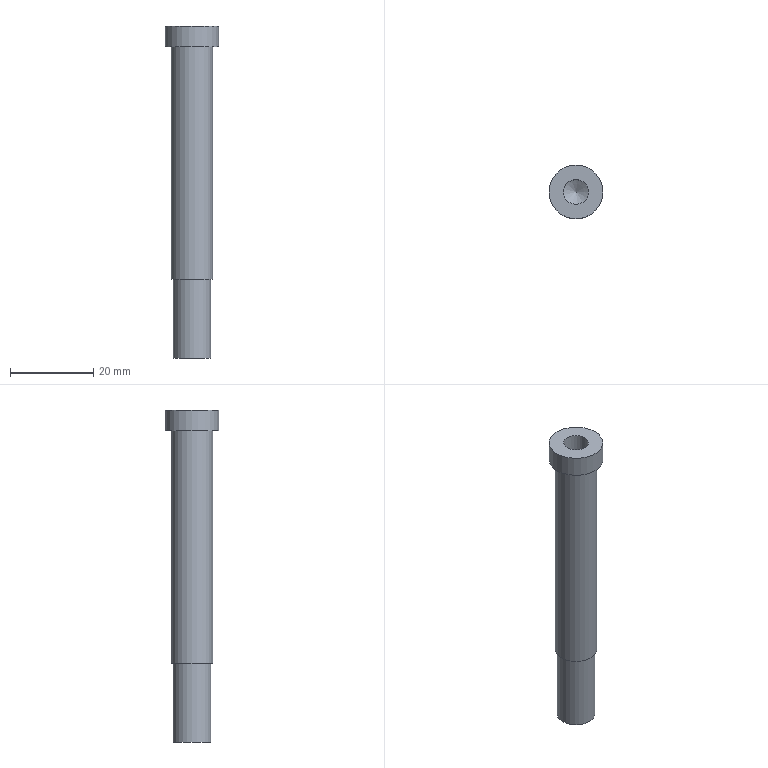Part | NX | features solid 2 | 1 solid | 9 faces | box 13 x 13 x 80 mm | volume 5914 mm3 | cylinder 4 | plane 4 | cone 1 | commonest cylinder face diameters 6 x1 9.1 x1 10 x1 13 x1
STEP:
#1=CARTESIAN_POINT('',(-691.699,-242.049,44.));
#2=VERTEX_POINT('',#1);
#3=CARTESIAN_POINT('',(-696.699,-242.049,44.));
#4=DIRECTION('',(0.,0.,1.));
#5=DIRECTION('',(1.,0.,0.));
#6=AXIS2_PLACEMENT_3D('',#3,#4,#5);
#7=CIRCLE('',#6,5.);
#8=EDGE_CURVE('',#2,#2,#7,.T.);
#9=ORIENTED_EDGE('',*,*,#8,.T.);
#10=EDGE_LOOP('',(#9));
#11=FACE_BOUND('',#10,.T.);
#12=CARTESIAN_POINT('',(-691.699,-242.049,100.));
#13=VERTEX_POINT('',#12);
#14=CARTESIAN_POINT('',(-696.699,-242.049,100.));
#15=DIRECTION('',(0.,0.,1.));
#16=DIRECTION('',(1.,0.,0.));
#17=AXIS2_PLACEMENT_3D('',#14,#15,#16);
#18=CIRCLE('',#17,5.);
#19=EDGE_CURVE('',#13,#13,#18,.T.);
#20=ORIENTED_EDGE('',*,*,#19,.F.);
#21=EDGE_LOOP('',(#20));
#22=FACE_BOUND('',#21,.T.);
#23=CARTESIAN_POINT('',(-696.699,-242.049,105.));
#24=DIRECTION('',(0.,0.,-1.));
#25=DIRECTION('',(-1.,0.,0.));
#26=AXIS2_PLACEMENT_3D('',#23,#24,#25);
#27=CYLINDRICAL_SURFACE('',#26,5.);
#28=ADVANCED_FACE('',(#11,#22),#27,.T.);
#29=CARTESIAN_POINT('',(-692.149,-242.049,44.));
#30=VERTEX_POINT('',#29);
#31=CARTESIAN_POINT('',(-696.699,-242.049,44.));
#32=DIRECTION('',(0.,0.,1.));
#33=DIRECTION('',(1.,0.,0.));
#34=AXIS2_PLACEMENT_3D('',#31,#32,#33);
#35=CIRCLE('',#34,4.55);
#36=EDGE_CURVE('',#30,#30,#35,.T.);
#37=ORIENTED_EDGE('',*,*,#36,.T.);
#38=EDGE_LOOP('',(#37));
#39=FACE_BOUND('',#38,.T.);
#40=ORIENTED_EDGE('',*,*,#8,.F.);
#41=EDGE_LOOP('',(#40));
#42=FACE_BOUND('',#41,.T.);
#43=CARTESIAN_POINT('',(-696.699,-242.049,44.));
#44=DIRECTION('',(0.,0.,1.));
#45=DIRECTION('',(1.,0.,0.));
#46=AXIS2_PLACEMENT_3D('',#43,#44,#45);
#47=PLANE('',#46);
#48=ADVANCED_FACE('',(#39,#42),#47,.F.);
#49=CARTESIAN_POINT('',(-690.199,-242.049,100.));
#50=VERTEX_POINT('',#49);
#51=CARTESIAN_POINT('',(-696.699,-242.049,100.));
#52=DIRECTION('',(0.,0.,1.));
#53=DIRECTION('',(1.,0.,0.));
#54=AXIS2_PLACEMENT_3D('',#51,#52,#53);
#55=CIRCLE('',#54,6.5);
#56=EDGE_CURVE('',#50,#50,#55,.T.);
#57=ORIENTED_EDGE('',*,*,#56,.F.);
#58=EDGE_LOOP('',(#57));
#59=FACE_BOUND('',#58,.T.);
#60=ORIENTED_EDGE('',*,*,#19,.T.);
#61=EDGE_LOOP('',(#60));
#62=FACE_BOUND('',#61,.T.);
#63=CARTESIAN_POINT('',(-696.699,-242.049,100.));
#64=DIRECTION('',(0.,0.,1.));
#65=DIRECTION('',(1.,0.,0.));
#66=AXIS2_PLACEMENT_3D('',#63,#64,#65);
#67=PLANE('',#66);
#68=ADVANCED_FACE('',(#59,#62),#67,.F.);
#69=ORIENTED_EDGE('',*,*,#56,.T.);
#70=EDGE_LOOP('',(#69));
#71=FACE_BOUND('',#70,.T.);
#72=CARTESIAN_POINT('',(-690.199,-242.049,105.));
#73=VERTEX_POINT('',#72);
#74=CARTESIAN_POINT('',(-696.699,-242.049,105.));
#75=DIRECTION('',(0.,0.,1.));
#76=DIRECTION('',(1.,0.,0.));
#77=AXIS2_PLACEMENT_3D('',#74,#75,#76);
#78=CIRCLE('',#77,6.5);
#79=EDGE_CURVE('',#73,#73,#78,.T.);
#80=ORIENTED_EDGE('',*,*,#79,.F.);
#81=EDGE_LOOP('',(#80));
#82=FACE_BOUND('',#81,.T.);
#83=CARTESIAN_POINT('',(-696.699,-242.049,100.));
#84=DIRECTION('',(0.,0.,1.));
#85=DIRECTION('',(1.,0.,0.));
#86=AXIS2_PLACEMENT_3D('',#83,#84,#85);
#87=CYLINDRICAL_SURFACE('',#86,6.5);
#88=ADVANCED_FACE('',(#71,#82),#87,.T.);
#89=CARTESIAN_POINT('',(-699.699,-242.049,105.));
#90=VERTEX_POINT('',#89);
#91=CARTESIAN_POINT('',(-696.699,-242.049,105.));
#92=DIRECTION('',(0.,0.,-1.));
#93=DIRECTION('',(-1.,0.,0.));
#94=AXIS2_PLACEMENT_3D('',#91,#92,#93);
#95=CIRCLE('',#94,3.);
#96=EDGE_CURVE('',#90,#90,#95,.T.);
#97=ORIENTED_EDGE('',*,*,#96,.T.);
#98=EDGE_LOOP('',(#97));
#99=FACE_BOUND('',#98,.T.);
#100=ORIENTED_EDGE('',*,*,#79,.T.);
#101=EDGE_LOOP('',(#100));
#102=FACE_BOUND('',#101,.T.);
#103=CARTESIAN_POINT('',(-696.699,-242.049,105.));
#104=DIRECTION('',(0.,0.,1.));
#105=DIRECTION('',(1.,0.,0.));
#106=AXIS2_PLACEMENT_3D('',#103,#104,#105);
#107=PLANE('',#106);
#108=ADVANCED_FACE('',(#99,#102),#107,.T.);
#109=CARTESIAN_POINT('',(-692.149,-242.049,25.));
#110=VERTEX_POINT('',#109);
#111=CARTESIAN_POINT('',(-696.699,-242.049,25.));
#112=DIRECTION('',(0.,0.,1.));
#113=DIRECTION('',(1.,0.,0.));
#114=AXIS2_PLACEMENT_3D('',#111,#112,#113);
#115=CIRCLE('',#114,4.55);
#116=EDGE_CURVE('',#110,#110,#115,.T.);
#117=ORIENTED_EDGE('',*,*,#116,.T.);
#118=EDGE_LOOP('',(#117));
#119=FACE_BOUND('',#118,.T.);
#120=ORIENTED_EDGE('',*,*,#36,.F.);
#121=EDGE_LOOP('',(#120));
#122=FACE_BOUND('',#121,.T.);
#123=CARTESIAN_POINT('',(-696.699,-242.049,25.));
#124=DIRECTION('',(0.,0.,1.));
#125=DIRECTION('',(1.,0.,0.));
#126=AXIS2_PLACEMENT_3D('',#123,#124,#125);
#127=CYLINDRICAL_SURFACE('',#126,4.55);
#128=ADVANCED_FACE('',(#119,#122),#127,.T.);
#129=ORIENTED_EDGE('',*,*,#116,.F.);
#130=EDGE_LOOP('',(#129));
#131=FACE_BOUND('',#130,.T.);
#132=CARTESIAN_POINT('',(-696.699,-242.049,25.));
#133=DIRECTION('',(0.,0.,1.));
#134=DIRECTION('',(1.,0.,0.));
#135=AXIS2_PLACEMENT_3D('',#132,#133,#134);
#136=PLANE('',#135);
#137=ADVANCED_FACE('',(#131),#136,.F.);
#138=CARTESIAN_POINT('',(-699.699,-242.049,92.));
#139=VERTEX_POINT('',#138);
#140=CARTESIAN_POINT('',(-696.699,-242.049,92.));
#141=DIRECTION('',(0.,0.,-1.));
#142=DIRECTION('',(-1.,0.,0.));
#143=AXIS2_PLACEMENT_3D('',#140,#141,#142);
#144=CIRCLE('',#143,3.);
#145=EDGE_CURVE('',#139,#139,#144,.T.);
#146=ORIENTED_EDGE('',*,*,#145,.F.);
#147=EDGE_LOOP('',(#146));
#148=FACE_BOUND('',#147,.T.);
#149=CARTESIAN_POINT('',(-696.699,-242.049,90.268));
#150=VERTEX_POINT('',#149);
#151=VERTEX_LOOP('',#150);
#152=FACE_BOUND('',#151,.T.);
#153=CARTESIAN_POINT('',(-696.699,-242.049,92.));
#154=DIRECTION('',(0.,0.,1.));
#155=DIRECTION('',(1.,0.,0.));
#156=AXIS2_PLACEMENT_3D('',#153,#154,#155);
#157=CONICAL_SURFACE('',#156,3.,1.047);
#158=ADVANCED_FACE('',(#148,#152),#157,.F.);
#159=ORIENTED_EDGE('',*,*,#145,.T.);
#160=EDGE_LOOP('',(#159));
#161=FACE_BOUND('',#160,.T.);
#162=ORIENTED_EDGE('',*,*,#96,.F.);
#163=EDGE_LOOP('',(#162));
#164=FACE_BOUND('',#163,.T.);
#165=CARTESIAN_POINT('',(-696.699,-242.049,105.));
#166=DIRECTION('',(0.,0.,-1.));
#167=DIRECTION('',(-1.,0.,0.));
#168=AXIS2_PLACEMENT_3D('',#165,#166,#167);
#169=CYLINDRICAL_SURFACE('',#168,3.);
#170=ADVANCED_FACE('',(#161,#164),#169,.F.);
#171=CLOSED_SHELL('',(#28,#48,#68,#88,#108,#128,#137,#158,#170));
#172=MANIFOLD_SOLID_BREP('',#171);
#173=(LENGTH_UNIT()NAMED_UNIT(*)SI_UNIT(.MILLI.,.METRE.));
#174=UNCERTAINTY_MEASURE_WITH_UNIT(LENGTH_MEASURE(0.00001),#173,'','');
#175=(NAMED_UNIT(*)PLANE_ANGLE_UNIT()SI_UNIT($,.RADIAN.));
#176=(NAMED_UNIT(*)SI_UNIT($,.STERADIAN.)SOLID_ANGLE_UNIT());
#177=(GEOMETRIC_REPRESENTATION_CONTEXT(3)GLOBAL_UNCERTAINTY_ASSIGNED_CONTEXT((#174))GLOBAL_UNIT_ASSIGNED_CONTEXT((#173,#175,#176))REPRESENTATION_CONTEXT('',''));
#178=ADVANCED_BREP_SHAPE_REPRESENTATION('',(#172),#177);